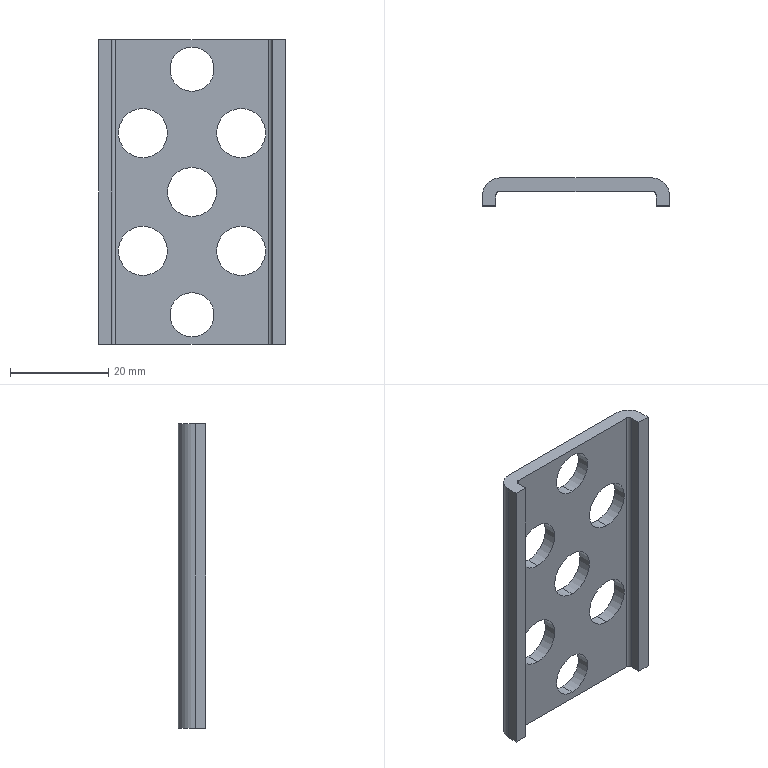Part | SolidWorks | features Fillet 2, HoleWzd 2, Extrusion 1, ICE 1 | 1 solid | 28 faces | box 37.996 x 5.595 x 62 mm | volume 5626 mm3 | cylinder 18 | plane 10 | commonest cylinder face diameters 10 x10 9 x4 1.473 x2 6.873 x2
STEP:
#1=CARTESIAN_POINT('',(0.,-2.7,-74.5));
#2=VERTEX_POINT('',#1);
#3=CARTESIAN_POINT('',(0.,-2.7,-65.5));
#4=VERTEX_POINT('',#3);
#5=CARTESIAN_POINT('',(0.,-2.7,-70.));
#6=DIRECTION('',(0.,1.,0.));
#7=DIRECTION('',(-1.,0.,0.));
#8=AXIS2_PLACEMENT_3D('',#5,#6,#7);
#9=CIRCLE('',#8,4.5);
#10=EDGE_CURVE('',#2,#4,#9,.T.);
#11=ORIENTED_EDGE('',*,*,#10,.F.);
#12=CARTESIAN_POINT('',(0.,0.,-74.5));
#13=VERTEX_POINT('',#12);
#14=CARTESIAN_POINT('',(0.,0.,-74.5));
#15=DIRECTION('',(0.,1.,0.));
#16=VECTOR('',#15,1000.);
#17=LINE('',#14,#16);
#18=EDGE_CURVE('',#2,#13,#17,.T.);
#19=ORIENTED_EDGE('',*,*,#18,.T.);
#20=CARTESIAN_POINT('',(0.,0.,-65.5));
#21=VERTEX_POINT('',#20);
#22=CARTESIAN_POINT('',(0.,0.,-70.));
#23=DIRECTION('',(0.,1.,0.));
#24=DIRECTION('',(0.,0.,1.));
#25=AXIS2_PLACEMENT_3D('',#22,#23,#24);
#26=CIRCLE('',#25,4.5);
#27=EDGE_CURVE('',#13,#21,#26,.T.);
#28=ORIENTED_EDGE('',*,*,#27,.T.);
#29=CARTESIAN_POINT('',(0.,0.,-65.5));
#30=DIRECTION('',(0.,1.,0.));
#31=VECTOR('',#30,1000.);
#32=LINE('',#29,#31);
#33=EDGE_CURVE('',#4,#21,#32,.T.);
#34=ORIENTED_EDGE('',*,*,#33,.F.);
#35=EDGE_LOOP('',(#11,#19,#28,#34));
#36=FACE_OUTER_BOUND('',#35,.T.);
#37=CARTESIAN_POINT('',(0.,0.,-70.));
#38=DIRECTION('',(0.,1.,0.));
#39=DIRECTION('',(0.,0.,1.));
#40=AXIS2_PLACEMENT_3D('',#37,#38,#39);
#41=CYLINDRICAL_SURFACE('',#40,4.5);
#42=ADVANCED_FACE('',(#36),#41,.F.);
#43=CARTESIAN_POINT('',(0.,-2.7,-24.5));
#44=VERTEX_POINT('',#43);
#45=CARTESIAN_POINT('',(0.,-2.7,-15.5));
#46=VERTEX_POINT('',#45);
#47=CARTESIAN_POINT('',(0.,-2.7,-20.));
#48=DIRECTION('',(0.,1.,0.));
#49=DIRECTION('',(-1.,0.,0.));
#50=AXIS2_PLACEMENT_3D('',#47,#48,#49);
#51=CIRCLE('',#50,4.5);
#52=EDGE_CURVE('',#44,#46,#51,.T.);
#53=ORIENTED_EDGE('',*,*,#52,.F.);
#54=CARTESIAN_POINT('',(0.,0.,-24.5));
#55=VERTEX_POINT('',#54);
#56=CARTESIAN_POINT('',(0.,0.,-24.5));
#57=DIRECTION('',(0.,1.,0.));
#58=VECTOR('',#57,1000.);
#59=LINE('',#56,#58);
#60=EDGE_CURVE('',#44,#55,#59,.T.);
#61=ORIENTED_EDGE('',*,*,#60,.T.);
#62=CARTESIAN_POINT('',(0.,0.,-15.5));
#63=VERTEX_POINT('',#62);
#64=CARTESIAN_POINT('',(0.,0.,-20.));
#65=DIRECTION('',(0.,1.,0.));
#66=DIRECTION('',(0.,0.,1.));
#67=AXIS2_PLACEMENT_3D('',#64,#65,#66);
#68=CIRCLE('',#67,4.5);
#69=EDGE_CURVE('',#55,#63,#68,.T.);
#70=ORIENTED_EDGE('',*,*,#69,.T.);
#71=CARTESIAN_POINT('',(0.,0.,-15.5));
#72=DIRECTION('',(0.,1.,0.));
#73=VECTOR('',#72,1000.);
#74=LINE('',#71,#73);
#75=EDGE_CURVE('',#46,#63,#74,.T.);
#76=ORIENTED_EDGE('',*,*,#75,.F.);
#77=EDGE_LOOP('',(#53,#61,#70,#76));
#78=FACE_OUTER_BOUND('',#77,.T.);
#79=CARTESIAN_POINT('',(0.,0.,-20.));
#80=DIRECTION('',(0.,1.,0.));
#81=DIRECTION('',(0.,0.,1.));
#82=AXIS2_PLACEMENT_3D('',#79,#80,#81);
#83=CYLINDRICAL_SURFACE('',#82,4.5);
#84=ADVANCED_FACE('',(#78),#83,.F.);
#85=CARTESIAN_POINT('',(0.,-2.7,-50.));
#86=VERTEX_POINT('',#85);
#87=CARTESIAN_POINT('',(0.,-2.7,-40.));
#88=VERTEX_POINT('',#87);
#89=CARTESIAN_POINT('',(0.,-2.7,-45.));
#90=DIRECTION('',(0.,1.,0.));
#91=DIRECTION('',(-1.,0.,0.));
#92=AXIS2_PLACEMENT_3D('',#89,#90,#91);
#93=CIRCLE('',#92,5.);
#94=EDGE_CURVE('',#86,#88,#93,.T.);
#95=ORIENTED_EDGE('',*,*,#94,.F.);
#96=CARTESIAN_POINT('',(0.,0.,-50.));
#97=VERTEX_POINT('',#96);
#98=CARTESIAN_POINT('',(0.,0.,-50.));
#99=DIRECTION('',(0.,1.,0.));
#100=VECTOR('',#99,1000.);
#101=LINE('',#98,#100);
#102=EDGE_CURVE('',#86,#97,#101,.T.);
#103=ORIENTED_EDGE('',*,*,#102,.T.);
#104=CARTESIAN_POINT('',(0.,0.,-40.));
#105=VERTEX_POINT('',#104);
#106=CARTESIAN_POINT('',(0.,0.,-45.));
#107=DIRECTION('',(0.,1.,0.));
#108=DIRECTION('',(0.,0.,1.));
#109=AXIS2_PLACEMENT_3D('',#106,#107,#108);
#110=CIRCLE('',#109,5.);
#111=EDGE_CURVE('',#97,#105,#110,.T.);
#112=ORIENTED_EDGE('',*,*,#111,.T.);
#113=CARTESIAN_POINT('',(0.,0.,-40.));
#114=DIRECTION('',(0.,1.,0.));
#115=VECTOR('',#114,1000.);
#116=LINE('',#113,#115);
#117=EDGE_CURVE('',#88,#105,#116,.T.);
#118=ORIENTED_EDGE('',*,*,#117,.F.);
#119=EDGE_LOOP('',(#95,#103,#112,#118));
#120=FACE_OUTER_BOUND('',#119,.T.);
#121=CARTESIAN_POINT('',(0.,0.,-45.));
#122=DIRECTION('',(0.,1.,0.));
#123=DIRECTION('',(0.,0.,1.));
#124=AXIS2_PLACEMENT_3D('',#121,#122,#123);
#125=CYLINDRICAL_SURFACE('',#124,5.);
#126=ADVANCED_FACE('',(#120),#125,.F.);
#127=CARTESIAN_POINT('',(-10.,-2.7,-62.));
#128=VERTEX_POINT('',#127);
#129=CARTESIAN_POINT('',(-10.,-2.7,-52.));
#130=VERTEX_POINT('',#129);
#131=CARTESIAN_POINT('',(-10.,-2.7,-57.));
#132=DIRECTION('',(0.,1.,0.));
#133=DIRECTION('',(-1.,0.,0.));
#134=AXIS2_PLACEMENT_3D('',#131,#132,#133);
#135=CIRCLE('',#134,5.);
#136=EDGE_CURVE('',#128,#130,#135,.T.);
#137=ORIENTED_EDGE('',*,*,#136,.F.);
#138=CARTESIAN_POINT('',(-10.,0.,-62.));
#139=VERTEX_POINT('',#138);
#140=CARTESIAN_POINT('',(-10.,0.,-62.));
#141=DIRECTION('',(0.,1.,0.));
#142=VECTOR('',#141,1000.);
#143=LINE('',#140,#142);
#144=EDGE_CURVE('',#128,#139,#143,.T.);
#145=ORIENTED_EDGE('',*,*,#144,.T.);
#146=CARTESIAN_POINT('',(-10.,0.,-52.));
#147=VERTEX_POINT('',#146);
#148=CARTESIAN_POINT('',(-10.,0.,-57.));
#149=DIRECTION('',(0.,1.,0.));
#150=DIRECTION('',(0.,0.,1.));
#151=AXIS2_PLACEMENT_3D('',#148,#149,#150);
#152=CIRCLE('',#151,5.);
#153=EDGE_CURVE('',#139,#147,#152,.T.);
#154=ORIENTED_EDGE('',*,*,#153,.T.);
#155=CARTESIAN_POINT('',(-10.,0.,-52.));
#156=DIRECTION('',(0.,1.,0.));
#157=VECTOR('',#156,1000.);
#158=LINE('',#155,#157);
#159=EDGE_CURVE('',#130,#147,#158,.T.);
#160=ORIENTED_EDGE('',*,*,#159,.F.);
#161=EDGE_LOOP('',(#137,#145,#154,#160));
#162=FACE_OUTER_BOUND('',#161,.T.);
#163=CARTESIAN_POINT('',(-10.,0.,-57.));
#164=DIRECTION('',(0.,1.,0.));
#165=DIRECTION('',(0.,0.,1.));
#166=AXIS2_PLACEMENT_3D('',#163,#164,#165);
#167=CYLINDRICAL_SURFACE('',#166,5.);
#168=ADVANCED_FACE('',(#162),#167,.F.);
#169=CARTESIAN_POINT('',(-10.,-2.7,-38.));
#170=VERTEX_POINT('',#169);
#171=CARTESIAN_POINT('',(-10.,-2.7,-28.));
#172=VERTEX_POINT('',#171);
#173=CARTESIAN_POINT('',(-10.,-2.7,-33.));
#174=DIRECTION('',(0.,1.,0.));
#175=DIRECTION('',(-1.,0.,0.));
#176=AXIS2_PLACEMENT_3D('',#173,#174,#175);
#177=CIRCLE('',#176,5.);
#178=EDGE_CURVE('',#170,#172,#177,.T.);
#179=ORIENTED_EDGE('',*,*,#178,.F.);
#180=CARTESIAN_POINT('',(-10.,0.,-38.));
#181=VERTEX_POINT('',#180);
#182=CARTESIAN_POINT('',(-10.,0.,-38.));
#183=DIRECTION('',(0.,1.,0.));
#184=VECTOR('',#183,1000.);
#185=LINE('',#182,#184);
#186=EDGE_CURVE('',#170,#181,#185,.T.);
#187=ORIENTED_EDGE('',*,*,#186,.T.);
#188=CARTESIAN_POINT('',(-10.,0.,-28.));
#189=VERTEX_POINT('',#188);
#190=CARTESIAN_POINT('',(-10.,0.,-33.));
#191=DIRECTION('',(0.,1.,0.));
#192=DIRECTION('',(0.,0.,1.));
#193=AXIS2_PLACEMENT_3D('',#190,#191,#192);
#194=CIRCLE('',#193,5.);
#195=EDGE_CURVE('',#181,#189,#194,.T.);
#196=ORIENTED_EDGE('',*,*,#195,.T.);
#197=CARTESIAN_POINT('',(-10.,0.,-28.));
#198=DIRECTION('',(0.,1.,0.));
#199=VECTOR('',#198,1000.);
#200=LINE('',#197,#199);
#201=EDGE_CURVE('',#172,#189,#200,.T.);
#202=ORIENTED_EDGE('',*,*,#201,.F.);
#203=EDGE_LOOP('',(#179,#187,#196,#202));
#204=FACE_OUTER_BOUND('',#203,.T.);
#205=CARTESIAN_POINT('',(-10.,0.,-33.));
#206=DIRECTION('',(0.,1.,0.));
#207=DIRECTION('',(0.,0.,1.));
#208=AXIS2_PLACEMENT_3D('',#205,#206,#207);
#209=CYLINDRICAL_SURFACE('',#208,5.);
#210=ADVANCED_FACE('',(#204),#209,.F.);
#211=CARTESIAN_POINT('',(10.,-2.7,-38.));
#212=VERTEX_POINT('',#211);
#213=CARTESIAN_POINT('',(10.,-2.7,-28.));
#214=VERTEX_POINT('',#213);
#215=CARTESIAN_POINT('',(10.,-2.7,-33.));
#216=DIRECTION('',(0.,1.,0.));
#217=DIRECTION('',(-1.,0.,0.));
#218=AXIS2_PLACEMENT_3D('',#215,#216,#217);
#219=CIRCLE('',#218,5.);
#220=EDGE_CURVE('',#212,#214,#219,.T.);
#221=ORIENTED_EDGE('',*,*,#220,.F.);
#222=CARTESIAN_POINT('',(10.,0.,-38.));
#223=VERTEX_POINT('',#222);
#224=CARTESIAN_POINT('',(10.,0.,-38.));
#225=DIRECTION('',(0.,1.,0.));
#226=VECTOR('',#225,1000.);
#227=LINE('',#224,#226);
#228=EDGE_CURVE('',#212,#223,#227,.T.);
#229=ORIENTED_EDGE('',*,*,#228,.T.);
#230=CARTESIAN_POINT('',(10.,0.,-28.));
#231=VERTEX_POINT('',#230);
#232=CARTESIAN_POINT('',(10.,0.,-33.));
#233=DIRECTION('',(0.,1.,0.));
#234=DIRECTION('',(0.,0.,1.));
#235=AXIS2_PLACEMENT_3D('',#232,#233,#234);
#236=CIRCLE('',#235,5.);
#237=EDGE_CURVE('',#223,#231,#236,.T.);
#238=ORIENTED_EDGE('',*,*,#237,.T.);
#239=CARTESIAN_POINT('',(10.,0.,-28.));
#240=DIRECTION('',(0.,1.,0.));
#241=VECTOR('',#240,1000.);
#242=LINE('',#239,#241);
#243=EDGE_CURVE('',#214,#231,#242,.T.);
#244=ORIENTED_EDGE('',*,*,#243,.F.);
#245=EDGE_LOOP('',(#221,#229,#238,#244));
#246=FACE_OUTER_BOUND('',#245,.T.);
#247=CARTESIAN_POINT('',(10.,0.,-33.));
#248=DIRECTION('',(0.,1.,0.));
#249=DIRECTION('',(0.,0.,1.));
#250=AXIS2_PLACEMENT_3D('',#247,#248,#249);
#251=CYLINDRICAL_SURFACE('',#250,5.);
#252=ADVANCED_FACE('',(#246),#251,.F.);
#253=CARTESIAN_POINT('',(10.,-2.7,-62.));
#254=VERTEX_POINT('',#253);
#255=CARTESIAN_POINT('',(10.,-2.7,-52.));
#256=VERTEX_POINT('',#255);
#257=CARTESIAN_POINT('',(10.,-2.7,-57.));
#258=DIRECTION('',(0.,1.,0.));
#259=DIRECTION('',(-1.,0.,0.));
#260=AXIS2_PLACEMENT_3D('',#257,#258,#259);
#261=CIRCLE('',#260,5.);
#262=EDGE_CURVE('',#254,#256,#261,.T.);
#263=ORIENTED_EDGE('',*,*,#262,.F.);
#264=CARTESIAN_POINT('',(10.,0.,-62.));
#265=VERTEX_POINT('',#264);
#266=CARTESIAN_POINT('',(10.,0.,-62.));
#267=DIRECTION('',(0.,1.,0.));
#268=VECTOR('',#267,1000.);
#269=LINE('',#266,#268);
#270=EDGE_CURVE('',#254,#265,#269,.T.);
#271=ORIENTED_EDGE('',*,*,#270,.T.);
#272=CARTESIAN_POINT('',(10.,0.,-52.));
#273=VERTEX_POINT('',#272);
#274=CARTESIAN_POINT('',(10.,0.,-57.));
#275=DIRECTION('',(0.,1.,0.));
#276=DIRECTION('',(0.,0.,1.));
#277=AXIS2_PLACEMENT_3D('',#274,#275,#276);
#278=CIRCLE('',#277,5.);
#279=EDGE_CURVE('',#265,#273,#278,.T.);
#280=ORIENTED_EDGE('',*,*,#279,.T.);
#281=CARTESIAN_POINT('',(10.,0.,-52.));
#282=DIRECTION('',(0.,1.,0.));
#283=VECTOR('',#282,1000.);
#284=LINE('',#281,#283);
#285=EDGE_CURVE('',#256,#273,#284,.T.);
#286=ORIENTED_EDGE('',*,*,#285,.F.);
#287=EDGE_LOOP('',(#263,#271,#280,#286));
#288=FACE_OUTER_BOUND('',#287,.T.);
#289=CARTESIAN_POINT('',(10.,0.,-57.));
#290=DIRECTION('',(0.,1.,0.));
#291=DIRECTION('',(0.,0.,1.));
#292=AXIS2_PLACEMENT_3D('',#289,#290,#291);
#293=CYLINDRICAL_SURFACE('',#292,5.);
#294=ADVANCED_FACE('',(#288),#293,.F.);
#295=CARTESIAN_POINT('',(16.298,-5.595,-14.));
#296=VERTEX_POINT('',#295);
#297=CARTESIAN_POINT('',(18.998,-5.595,-14.));
#298=VERTEX_POINT('',#297);
#299=CARTESIAN_POINT('',(-18.998,-5.595,-14.));
#300=DIRECTION('',(1.,0.,0.));
#301=VECTOR('',#300,1000.);
#302=LINE('',#299,#301);
#303=EDGE_CURVE('',#296,#298,#302,.T.);
#304=ORIENTED_EDGE('',*,*,#303,.F.);
#305=CARTESIAN_POINT('',(16.298,-5.595,-76.));
#306=VERTEX_POINT('',#305);
#307=CARTESIAN_POINT('',(16.298,-5.595,-14.));
#308=DIRECTION('',(0.,0.,-1.));
#309=VECTOR('',#308,1000.);
#310=LINE('',#307,#309);
#311=EDGE_CURVE('',#296,#306,#310,.T.);
#312=ORIENTED_EDGE('',*,*,#311,.T.);
#313=CARTESIAN_POINT('',(18.998,-5.595,-76.));
#314=VERTEX_POINT('',#313);
#315=CARTESIAN_POINT('',(18.998,-5.595,-76.));
#316=DIRECTION('',(-1.,0.,0.));
#317=VECTOR('',#316,1000.);
#318=LINE('',#315,#317);
#319=EDGE_CURVE('',#314,#306,#318,.T.);
#320=ORIENTED_EDGE('',*,*,#319,.F.);
#321=CARTESIAN_POINT('',(18.998,-5.595,-14.));
#322=DIRECTION('',(0.,0.,-1.));
#323=VECTOR('',#322,1000.);
#324=LINE('',#321,#323);
#325=EDGE_CURVE('',#298,#314,#324,.T.);
#326=ORIENTED_EDGE('',*,*,#325,.F.);
#327=EDGE_LOOP('',(#304,#312,#320,#326));
#328=FACE_OUTER_BOUND('',#327,.T.);
#329=CARTESIAN_POINT('',(0.,-5.595,0.));
#330=DIRECTION('',(0.,1.,0.));
#331=DIRECTION('',(0.,0.,1.));
#332=AXIS2_PLACEMENT_3D('',#329,#330,#331);
#333=PLANE('',#332);
#334=ADVANCED_FACE('',(#328),#333,.F.);
#335=CARTESIAN_POINT('',(-18.998,-5.595,-14.));
#336=VERTEX_POINT('',#335);
#337=CARTESIAN_POINT('',(-18.998,-3.437,-14.));
#338=VERTEX_POINT('',#337);
#339=CARTESIAN_POINT('',(-18.998,-5.595,-14.));
#340=DIRECTION('',(0.,1.,0.));
#341=VECTOR('',#340,1000.);
#342=LINE('',#339,#341);
#343=EDGE_CURVE('',#336,#338,#342,.T.);
#344=ORIENTED_EDGE('',*,*,#343,.T.);
#345=CARTESIAN_POINT('',(-18.998,-3.437,-76.));
#346=VERTEX_POINT('',#345);
#347=CARTESIAN_POINT('',(-18.998,-3.437,-76.));
#348=DIRECTION('',(0.,0.,-1.));
#349=VECTOR('',#348,1000.);
#350=LINE('',#347,#349);
#351=EDGE_CURVE('',#338,#346,#350,.T.);
#352=ORIENTED_EDGE('',*,*,#351,.T.);
#353=CARTESIAN_POINT('',(-18.998,-5.595,-76.));
#354=VERTEX_POINT('',#353);
#355=CARTESIAN_POINT('',(-18.998,-5.595,-76.));
#356=DIRECTION('',(0.,1.,0.));
#357=VECTOR('',#356,1000.);
#358=LINE('',#355,#357);
#359=EDGE_CURVE('',#354,#346,#358,.T.);
#360=ORIENTED_EDGE('',*,*,#359,.F.);
#361=CARTESIAN_POINT('',(-18.998,-5.595,-76.));
#362=DIRECTION('',(0.,0.,1.));
#363=VECTOR('',#362,1000.);
#364=LINE('',#361,#363);
#365=EDGE_CURVE('',#354,#336,#364,.T.);
#366=ORIENTED_EDGE('',*,*,#365,.T.);
#367=EDGE_LOOP('',(#344,#352,#360,#366));
#368=FACE_OUTER_BOUND('',#367,.T.);
#369=CARTESIAN_POINT('',(-18.998,-5.595,-76.));
#370=DIRECTION('',(-1.,0.,0.));
#371=DIRECTION('',(0.,0.,1.));
#372=AXIS2_PLACEMENT_3D('',#369,#370,#371);
#373=PLANE('',#372);
#374=ADVANCED_FACE('',(#368),#373,.T.);
#375=CARTESIAN_POINT('',(15.561,0.,-76.));
#376=VERTEX_POINT('',#375);
#377=CARTESIAN_POINT('',(-15.561,0.,-76.));
#378=VERTEX_POINT('',#377);
#379=CARTESIAN_POINT('',(18.998,0.,-76.));
#380=DIRECTION('',(-1.,0.,0.));
#381=VECTOR('',#380,1000.);
#382=LINE('',#379,#381);
#383=EDGE_CURVE('',#376,#378,#382,.T.);
#384=ORIENTED_EDGE('',*,*,#383,.F.);
#385=CARTESIAN_POINT('',(18.998,-3.437,-76.));
#386=VERTEX_POINT('',#385);
#387=CARTESIAN_POINT('',(15.561,-3.437,-76.));
#388=DIRECTION('',(0.,0.,-1.));
#389=DIRECTION('',(-1.,0.,0.));
#390=AXIS2_PLACEMENT_3D('',#387,#388,#389);
#391=CIRCLE('',#390,3.437);
#392=EDGE_CURVE('',#376,#386,#391,.T.);
#393=ORIENTED_EDGE('',*,*,#392,.T.);
#394=CARTESIAN_POINT('',(18.998,-5.595,-76.));
#395=DIRECTION('',(0.,1.,0.));
#396=VECTOR('',#395,1000.);
#397=LINE('',#394,#396);
#398=EDGE_CURVE('',#314,#386,#397,.T.);
#399=ORIENTED_EDGE('',*,*,#398,.F.);
#400=ORIENTED_EDGE('',*,*,#319,.T.);
#401=CARTESIAN_POINT('',(16.298,-3.437,-76.));
#402=VERTEX_POINT('',#401);
#403=CARTESIAN_POINT('',(16.298,-2.7,-76.));
#404=DIRECTION('',(0.,-1.,0.));
#405=VECTOR('',#404,1000.);
#406=LINE('',#403,#405);
#407=EDGE_CURVE('',#402,#306,#406,.T.);
#408=ORIENTED_EDGE('',*,*,#407,.F.);
#409=CARTESIAN_POINT('',(15.561,-2.7,-76.));
#410=VERTEX_POINT('',#409);
#411=CARTESIAN_POINT('',(15.561,-3.437,-76.));
#412=DIRECTION('',(0.,0.,1.));
#413=DIRECTION('',(-1.,0.,0.));
#414=AXIS2_PLACEMENT_3D('',#411,#412,#413);
#415=CIRCLE('',#414,0.7366);
#416=EDGE_CURVE('',#402,#410,#415,.T.);
#417=ORIENTED_EDGE('',*,*,#416,.T.);
#418=CARTESIAN_POINT('',(-15.561,-2.7,-76.));
#419=VERTEX_POINT('',#418);
#420=CARTESIAN_POINT('',(-16.298,-2.7,-76.));
#421=DIRECTION('',(1.,0.,0.));
#422=VECTOR('',#421,1000.);
#423=LINE('',#420,#422);
#424=EDGE_CURVE('',#419,#410,#423,.T.);
#425=ORIENTED_EDGE('',*,*,#424,.F.);
#426=CARTESIAN_POINT('',(-16.298,-3.437,-76.));
#427=VERTEX_POINT('',#426);
#428=CARTESIAN_POINT('',(-15.561,-3.437,-76.));
#429=DIRECTION('',(0.,0.,1.));
#430=DIRECTION('',(-1.,0.,0.));
#431=AXIS2_PLACEMENT_3D('',#428,#429,#430);
#432=CIRCLE('',#431,0.7366);
#433=EDGE_CURVE('',#419,#427,#432,.T.);
#434=ORIENTED_EDGE('',*,*,#433,.T.);
#435=CARTESIAN_POINT('',(-16.298,-5.595,-76.));
#436=VERTEX_POINT('',#435);
#437=CARTESIAN_POINT('',(-16.298,-5.595,-76.));
#438=DIRECTION('',(0.,1.,0.));
#439=VECTOR('',#438,1000.);
#440=LINE('',#437,#439);
#441=EDGE_CURVE('',#436,#427,#440,.T.);
#442=ORIENTED_EDGE('',*,*,#441,.F.);
#443=CARTESIAN_POINT('',(18.998,-5.595,-76.));
#444=DIRECTION('',(-1.,0.,0.));
#445=VECTOR('',#444,1000.);
#446=LINE('',#443,#445);
#447=EDGE_CURVE('',#436,#354,#446,.T.);
#448=ORIENTED_EDGE('',*,*,#447,.T.);
#449=ORIENTED_EDGE('',*,*,#359,.T.);
#450=CARTESIAN_POINT('',(-15.561,-3.437,-76.));
#451=DIRECTION('',(0.,0.,-1.));
#452=DIRECTION('',(-1.,0.,0.));
#453=AXIS2_PLACEMENT_3D('',#450,#451,#452);
#454=CIRCLE('',#453,3.437);
#455=EDGE_CURVE('',#346,#378,#454,.T.);
#456=ORIENTED_EDGE('',*,*,#455,.T.);
#457=EDGE_LOOP('',(#384,#393,#399,#400,#408,#417,#425,#434,#442,#448,#449,#456));
#458=FACE_OUTER_BOUND('',#457,.T.);
#459=CARTESIAN_POINT('',(18.998,-5.595,-76.));
#460=DIRECTION('',(0.,0.,-1.));
#461=DIRECTION('',(-1.,0.,0.));
#462=AXIS2_PLACEMENT_3D('',#459,#460,#461);
#463=PLANE('',#462);
#464=ADVANCED_FACE('',(#458),#463,.T.);
#465=ORIENTED_EDGE('',*,*,#398,.T.);
#466=CARTESIAN_POINT('',(18.998,-3.437,-14.));
#467=VERTEX_POINT('',#466);
#468=CARTESIAN_POINT('',(18.998,-3.437,-14.));
#469=DIRECTION('',(0.,0.,1.));
#470=VECTOR('',#469,1000.);
#471=LINE('',#468,#470);
#472=EDGE_CURVE('',#386,#467,#471,.T.);
#473=ORIENTED_EDGE('',*,*,#472,.T.);
#474=CARTESIAN_POINT('',(18.998,-5.595,-14.));
#475=DIRECTION('',(0.,1.,0.));
#476=VECTOR('',#475,1000.);
#477=LINE('',#474,#476);
#478=EDGE_CURVE('',#298,#467,#477,.T.);
#479=ORIENTED_EDGE('',*,*,#478,.F.);
#480=ORIENTED_EDGE('',*,*,#325,.T.);
#481=EDGE_LOOP('',(#465,#473,#479,#480));
#482=FACE_OUTER_BOUND('',#481,.T.);
#483=CARTESIAN_POINT('',(18.998,-5.595,-14.));
#484=DIRECTION('',(1.,0.,0.));
#485=DIRECTION('',(0.,0.,-1.));
#486=AXIS2_PLACEMENT_3D('',#483,#484,#485);
#487=PLANE('',#486);
#488=ADVANCED_FACE('',(#482),#487,.T.);
#489=ORIENTED_EDGE('',*,*,#478,.T.);
#490=CARTESIAN_POINT('',(15.561,0.,-14.));
#491=VERTEX_POINT('',#490);
#492=CARTESIAN_POINT('',(15.561,-3.437,-14.));
#493=DIRECTION('',(0.,0.,1.));
#494=DIRECTION('',(1.,0.,0.));
#495=AXIS2_PLACEMENT_3D('',#492,#493,#494);
#496=CIRCLE('',#495,3.437);
#497=EDGE_CURVE('',#467,#491,#496,.T.);
#498=ORIENTED_EDGE('',*,*,#497,.T.);
#499=CARTESIAN_POINT('',(-15.561,0.,-14.));
#500=VERTEX_POINT('',#499);
#501=CARTESIAN_POINT('',(-18.998,0.,-14.));
#502=DIRECTION('',(1.,0.,0.));
#503=VECTOR('',#502,1000.);
#504=LINE('',#501,#503);
#505=EDGE_CURVE('',#500,#491,#504,.T.);
#506=ORIENTED_EDGE('',*,*,#505,.F.);
#507=CARTESIAN_POINT('',(-15.561,-3.437,-14.));
#508=DIRECTION('',(0.,0.,1.));
#509=DIRECTION('',(1.,0.,0.));
#510=AXIS2_PLACEMENT_3D('',#507,#508,#509);
#511=CIRCLE('',#510,3.437);
#512=EDGE_CURVE('',#500,#338,#511,.T.);
#513=ORIENTED_EDGE('',*,*,#512,.T.);
#514=ORIENTED_EDGE('',*,*,#343,.F.);
#515=CARTESIAN_POINT('',(-16.298,-5.595,-14.));
#516=VERTEX_POINT('',#515);
#517=CARTESIAN_POINT('',(-18.998,-5.595,-14.));
#518=DIRECTION('',(1.,0.,0.));
#519=VECTOR('',#518,1000.);
#520=LINE('',#517,#519);
#521=EDGE_CURVE('',#336,#516,#520,.T.);
#522=ORIENTED_EDGE('',*,*,#521,.T.);
#523=CARTESIAN_POINT('',(-16.298,-3.437,-14.));
#524=VERTEX_POINT('',#523);
#525=CARTESIAN_POINT('',(-16.298,-5.595,-14.));
#526=DIRECTION('',(0.,1.,0.));
#527=VECTOR('',#526,1000.);
#528=LINE('',#525,#527);
#529=EDGE_CURVE('',#516,#524,#528,.T.);
#530=ORIENTED_EDGE('',*,*,#529,.T.);
#531=CARTESIAN_POINT('',(-15.561,-2.7,-14.));
#532=VERTEX_POINT('',#531);
#533=CARTESIAN_POINT('',(-15.561,-3.437,-14.));
#534=DIRECTION('',(0.,0.,-1.));
#535=DIRECTION('',(1.,0.,0.));
#536=AXIS2_PLACEMENT_3D('',#533,#534,#535);
#537=CIRCLE('',#536,0.7366);
#538=EDGE_CURVE('',#524,#532,#537,.T.);
#539=ORIENTED_EDGE('',*,*,#538,.T.);
#540=CARTESIAN_POINT('',(15.561,-2.7,-14.));
#541=VERTEX_POINT('',#540);
#542=CARTESIAN_POINT('',(-16.298,-2.7,-14.));
#543=DIRECTION('',(1.,0.,0.));
#544=VECTOR('',#543,1000.);
#545=LINE('',#542,#544);
#546=EDGE_CURVE('',#532,#541,#545,.T.);
#547=ORIENTED_EDGE('',*,*,#546,.T.);
#548=CARTESIAN_POINT('',(16.298,-3.437,-14.));
#549=VERTEX_POINT('',#548);
#550=CARTESIAN_POINT('',(15.561,-3.437,-14.));
#551=DIRECTION('',(0.,0.,-1.));
#552=DIRECTION('',(1.,0.,0.));
#553=AXIS2_PLACEMENT_3D('',#550,#551,#552);
#554=CIRCLE('',#553,0.7366);
#555=EDGE_CURVE('',#541,#549,#554,.T.);
#556=ORIENTED_EDGE('',*,*,#555,.T.);
#557=CARTESIAN_POINT('',(16.298,-2.7,-14.));
#558=DIRECTION('',(0.,-1.,0.));
#559=VECTOR('',#558,1000.);
#560=LINE('',#557,#559);
#561=EDGE_CURVE('',#549,#296,#560,.T.);
#562=ORIENTED_EDGE('',*,*,#561,.T.);
#563=ORIENTED_EDGE('',*,*,#303,.T.);
#564=EDGE_LOOP('',(#489,#498,#506,#513,#514,#522,#530,#539,#547,#556,#562,#563));
#565=FACE_OUTER_BOUND('',#564,.T.);
#566=CARTESIAN_POINT('',(-18.998,-5.595,-14.));
#567=DIRECTION('',(0.,0.,1.));
#568=DIRECTION('',(1.,0.,0.));
#569=AXIS2_PLACEMENT_3D('',#566,#567,#568);
#570=PLANE('',#569);
#571=ADVANCED_FACE('',(#565),#570,.T.);
#572=ORIENTED_EDGE('',*,*,#447,.F.);
#573=CARTESIAN_POINT('',(-16.298,-5.595,-14.));
#574=DIRECTION('',(0.,0.,-1.));
#575=VECTOR('',#574,1000.);
#576=LINE('',#573,#575);
#577=EDGE_CURVE('',#516,#436,#576,.T.);
#578=ORIENTED_EDGE('',*,*,#577,.F.);
#579=ORIENTED_EDGE('',*,*,#521,.F.);
#580=ORIENTED_EDGE('',*,*,#365,.F.);
#581=EDGE_LOOP('',(#572,#578,#579,#580));
#582=FACE_OUTER_BOUND('',#581,.T.);
#583=CARTESIAN_POINT('',(0.,-5.595,0.));
#584=DIRECTION('',(0.,1.,0.));
#585=DIRECTION('',(0.,0.,1.));
#586=AXIS2_PLACEMENT_3D('',#583,#584,#585);
#587=PLANE('',#586);
#588=ADVANCED_FACE('',(#582),#587,.F.);
#589=CARTESIAN_POINT('',(0.,0.,-70.));
#590=DIRECTION('',(0.,1.,0.));
#591=DIRECTION('',(0.,0.,1.));
#592=AXIS2_PLACEMENT_3D('',#589,#590,#591);
#593=CIRCLE('',#592,4.5);
#594=EDGE_CURVE('',#21,#13,#593,.T.);
#595=ORIENTED_EDGE('',*,*,#594,.F.);
#596=ORIENTED_EDGE('',*,*,#27,.F.);
#597=EDGE_LOOP('',(#595,#596));
#598=FACE_BOUND('',#597,.T.);
#599=CARTESIAN_POINT('',(0.,0.,-20.));
#600=DIRECTION('',(0.,1.,0.));
#601=DIRECTION('',(0.,0.,1.));
#602=AXIS2_PLACEMENT_3D('',#599,#600,#601);
#603=CIRCLE('',#602,4.5);
#604=EDGE_CURVE('',#63,#55,#603,.T.);
#605=ORIENTED_EDGE('',*,*,#604,.F.);
#606=ORIENTED_EDGE('',*,*,#69,.F.);
#607=EDGE_LOOP('',(#605,#606));
#608=FACE_BOUND('',#607,.T.);
#609=CARTESIAN_POINT('',(0.,0.,-45.));
#610=DIRECTION('',(0.,1.,0.));
#611=DIRECTION('',(0.,0.,1.));
#612=AXIS2_PLACEMENT_3D('',#609,#610,#611);
#613=CIRCLE('',#612,5.);
#614=EDGE_CURVE('',#105,#97,#613,.T.);
#615=ORIENTED_EDGE('',*,*,#614,.F.);
#616=ORIENTED_EDGE('',*,*,#111,.F.);
#617=EDGE_LOOP('',(#615,#616));
#618=FACE_BOUND('',#617,.T.);
#619=CARTESIAN_POINT('',(-10.,0.,-57.));
#620=DIRECTION('',(0.,1.,0.));
#621=DIRECTION('',(0.,0.,1.));
#622=AXIS2_PLACEMENT_3D('',#619,#620,#621);
#623=CIRCLE('',#622,5.);
#624=EDGE_CURVE('',#147,#139,#623,.T.);
#625=ORIENTED_EDGE('',*,*,#624,.F.);
#626=ORIENTED_EDGE('',*,*,#153,.F.);
#627=EDGE_LOOP('',(#625,#626));
#628=FACE_BOUND('',#627,.T.);
#629=CARTESIAN_POINT('',(-10.,0.,-33.));
#630=DIRECTION('',(0.,1.,0.));
#631=DIRECTION('',(0.,0.,1.));
#632=AXIS2_PLACEMENT_3D('',#629,#630,#631);
#633=CIRCLE('',#632,5.);
#634=EDGE_CURVE('',#189,#181,#633,.T.);
#635=ORIENTED_EDGE('',*,*,#634,.F.);
#636=ORIENTED_EDGE('',*,*,#195,.F.);
#637=EDGE_LOOP('',(#635,#636));
#638=FACE_BOUND('',#637,.T.);
#639=CARTESIAN_POINT('',(10.,0.,-33.));
#640=DIRECTION('',(0.,1.,0.));
#641=DIRECTION('',(0.,0.,1.));
#642=AXIS2_PLACEMENT_3D('',#639,#640,#641);
#643=CIRCLE('',#642,5.);
#644=EDGE_CURVE('',#231,#223,#643,.T.);
#645=ORIENTED_EDGE('',*,*,#644,.F.);
#646=ORIENTED_EDGE('',*,*,#237,.F.);
#647=EDGE_LOOP('',(#645,#646));
#648=FACE_BOUND('',#647,.T.);
#649=CARTESIAN_POINT('',(10.,0.,-57.));
#650=DIRECTION('',(0.,1.,0.));
#651=DIRECTION('',(0.,0.,1.));
#652=AXIS2_PLACEMENT_3D('',#649,#650,#651);
#653=CIRCLE('',#652,5.);
#654=EDGE_CURVE('',#273,#265,#653,.T.);
#655=ORIENTED_EDGE('',*,*,#654,.F.);
#656=ORIENTED_EDGE('',*,*,#279,.F.);
#657=EDGE_LOOP('',(#655,#656));
#658=FACE_BOUND('',#657,.T.);
#659=ORIENTED_EDGE('',*,*,#505,.T.);
#660=CARTESIAN_POINT('',(15.561,0.,0.));
#661=DIRECTION('',(0.,0.,-1.));
#662=VECTOR('',#661,1000.);
#663=LINE('',#660,#662);
#664=EDGE_CURVE('',#491,#376,#663,.T.);
#665=ORIENTED_EDGE('',*,*,#664,.T.);
#666=ORIENTED_EDGE('',*,*,#383,.T.);
#667=CARTESIAN_POINT('',(-15.561,0.,0.));
#668=DIRECTION('',(0.,0.,1.));
#669=VECTOR('',#668,1000.);
#670=LINE('',#667,#669);
#671=EDGE_CURVE('',#378,#500,#670,.T.);
#672=ORIENTED_EDGE('',*,*,#671,.T.);
#673=EDGE_LOOP('',(#659,#665,#666,#672));
#674=FACE_OUTER_BOUND('',#673,.T.);
#675=CARTESIAN_POINT('',(0.,0.,0.));
#676=DIRECTION('',(0.,1.,0.));
#677=DIRECTION('',(0.,0.,1.));
#678=AXIS2_PLACEMENT_3D('',#675,#676,#677);
#679=PLANE('',#678);
#680=ADVANCED_FACE('',(#598,#608,#618,#628,#638,#648,#658,#674),#679,.T.);
#681=ORIENTED_EDGE('',*,*,#561,.F.);
#682=CARTESIAN_POINT('',(16.298,-3.437,-76.));
#683=DIRECTION('',(0.,0.,-1.));
#684=VECTOR('',#683,1000.);
#685=LINE('',#682,#684);
#686=EDGE_CURVE('',#549,#402,#685,.T.);
#687=ORIENTED_EDGE('',*,*,#686,.T.);
#688=ORIENTED_EDGE('',*,*,#407,.T.);
#689=ORIENTED_EDGE('',*,*,#311,.F.);
#690=EDGE_LOOP('',(#681,#687,#688,#689));
#691=FACE_OUTER_BOUND('',#690,.T.);
#692=CARTESIAN_POINT('',(16.298,-2.7,-14.));
#693=DIRECTION('',(1.,0.,0.));
#694=DIRECTION('',(0.,1.,0.));
#695=AXIS2_PLACEMENT_3D('',#692,#693,#694);
#696=PLANE('',#695);
#697=ADVANCED_FACE('',(#691),#696,.F.);
#698=CARTESIAN_POINT('',(0.,-2.7,-70.));
#699=DIRECTION('',(0.,1.,0.));
#700=DIRECTION('',(-1.,0.,0.));
#701=AXIS2_PLACEMENT_3D('',#698,#699,#700);
#702=CIRCLE('',#701,4.5);
#703=EDGE_CURVE('',#4,#2,#702,.T.);
#704=ORIENTED_EDGE('',*,*,#703,.T.);
#705=ORIENTED_EDGE('',*,*,#10,.T.);
#706=EDGE_LOOP('',(#704,#705));
#707=FACE_BOUND('',#706,.T.);
#708=CARTESIAN_POINT('',(0.,-2.7,-20.));
#709=DIRECTION('',(0.,1.,0.));
#710=DIRECTION('',(-1.,0.,0.));
#711=AXIS2_PLACEMENT_3D('',#708,#709,#710);
#712=CIRCLE('',#711,4.5);
#713=EDGE_CURVE('',#46,#44,#712,.T.);
#714=ORIENTED_EDGE('',*,*,#713,.T.);
#715=ORIENTED_EDGE('',*,*,#52,.T.);
#716=EDGE_LOOP('',(#714,#715));
#717=FACE_BOUND('',#716,.T.);
#718=CARTESIAN_POINT('',(0.,-2.7,-45.));
#719=DIRECTION('',(0.,1.,0.));
#720=DIRECTION('',(-1.,0.,0.));
#721=AXIS2_PLACEMENT_3D('',#718,#719,#720);
#722=CIRCLE('',#721,5.);
#723=EDGE_CURVE('',#88,#86,#722,.T.);
#724=ORIENTED_EDGE('',*,*,#723,.T.);
#725=ORIENTED_EDGE('',*,*,#94,.T.);
#726=EDGE_LOOP('',(#724,#725));
#727=FACE_BOUND('',#726,.T.);
#728=CARTESIAN_POINT('',(-10.,-2.7,-57.));
#729=DIRECTION('',(0.,1.,0.));
#730=DIRECTION('',(-1.,0.,0.));
#731=AXIS2_PLACEMENT_3D('',#728,#729,#730);
#732=CIRCLE('',#731,5.);
#733=EDGE_CURVE('',#130,#128,#732,.T.);
#734=ORIENTED_EDGE('',*,*,#733,.T.);
#735=ORIENTED_EDGE('',*,*,#136,.T.);
#736=EDGE_LOOP('',(#734,#735));
#737=FACE_BOUND('',#736,.T.);
#738=CARTESIAN_POINT('',(-10.,-2.7,-33.));
#739=DIRECTION('',(0.,1.,0.));
#740=DIRECTION('',(-1.,0.,0.));
#741=AXIS2_PLACEMENT_3D('',#738,#739,#740);
#742=CIRCLE('',#741,5.);
#743=EDGE_CURVE('',#172,#170,#742,.T.);
#744=ORIENTED_EDGE('',*,*,#743,.T.);
#745=ORIENTED_EDGE('',*,*,#178,.T.);
#746=EDGE_LOOP('',(#744,#745));
#747=FACE_BOUND('',#746,.T.);
#748=CARTESIAN_POINT('',(10.,-2.7,-33.));
#749=DIRECTION('',(0.,1.,0.));
#750=DIRECTION('',(-1.,0.,0.));
#751=AXIS2_PLACEMENT_3D('',#748,#749,#750);
#752=CIRCLE('',#751,5.);
#753=EDGE_CURVE('',#214,#212,#752,.T.);
#754=ORIENTED_EDGE('',*,*,#753,.T.);
#755=ORIENTED_EDGE('',*,*,#220,.T.);
#756=EDGE_LOOP('',(#754,#755));
#757=FACE_BOUND('',#756,.T.);
#758=CARTESIAN_POINT('',(10.,-2.7,-57.));
#759=DIRECTION('',(0.,1.,0.));
#760=DIRECTION('',(-1.,0.,0.));
#761=AXIS2_PLACEMENT_3D('',#758,#759,#760);
#762=CIRCLE('',#761,5.);
#763=EDGE_CURVE('',#256,#254,#762,.T.);
#764=ORIENTED_EDGE('',*,*,#763,.T.);
#765=ORIENTED_EDGE('',*,*,#262,.T.);
#766=EDGE_LOOP('',(#764,#765));
#767=FACE_BOUND('',#766,.T.);
#768=ORIENTED_EDGE('',*,*,#546,.F.);
#769=CARTESIAN_POINT('',(-15.561,-2.7,-76.));
#770=DIRECTION('',(0.,0.,-1.));
#771=VECTOR('',#770,1000.);
#772=LINE('',#769,#771);
#773=EDGE_CURVE('',#532,#419,#772,.T.);
#774=ORIENTED_EDGE('',*,*,#773,.T.);
#775=ORIENTED_EDGE('',*,*,#424,.T.);
#776=CARTESIAN_POINT('',(15.561,-2.7,-14.));
#777=DIRECTION('',(0.,0.,1.));
#778=VECTOR('',#777,1000.);
#779=LINE('',#776,#778);
#780=EDGE_CURVE('',#410,#541,#779,.T.);
#781=ORIENTED_EDGE('',*,*,#780,.T.);
#782=EDGE_LOOP('',(#768,#774,#775,#781));
#783=FACE_OUTER_BOUND('',#782,.T.);
#784=CARTESIAN_POINT('',(-16.298,-2.7,-14.));
#785=DIRECTION('',(0.,1.,0.));
#786=DIRECTION('',(-1.,0.,0.));
#787=AXIS2_PLACEMENT_3D('',#784,#785,#786);
#788=PLANE('',#787);
#789=ADVANCED_FACE('',(#707,#717,#727,#737,#747,#757,#767,#783),#788,.F.);
#790=ORIENTED_EDGE('',*,*,#441,.T.);
#791=CARTESIAN_POINT('',(-16.298,-3.437,-14.));
#792=DIRECTION('',(0.,0.,1.));
#793=VECTOR('',#792,1000.);
#794=LINE('',#791,#793);
#795=EDGE_CURVE('',#427,#524,#794,.T.);
#796=ORIENTED_EDGE('',*,*,#795,.T.);
#797=ORIENTED_EDGE('',*,*,#529,.F.);
#798=ORIENTED_EDGE('',*,*,#577,.T.);
#799=EDGE_LOOP('',(#790,#796,#797,#798));
#800=FACE_OUTER_BOUND('',#799,.T.);
#801=CARTESIAN_POINT('',(-16.298,-5.595,-14.));
#802=DIRECTION('',(-1.,0.,0.));
#803=DIRECTION('',(0.,-1.,0.));
#804=AXIS2_PLACEMENT_3D('',#801,#802,#803);
#805=PLANE('',#804);
#806=ADVANCED_FACE('',(#800),#805,.F.);
#807=ORIENTED_EDGE('',*,*,#270,.F.);
#808=ORIENTED_EDGE('',*,*,#763,.F.);
#809=ORIENTED_EDGE('',*,*,#285,.T.);
#810=ORIENTED_EDGE('',*,*,#654,.T.);
#811=EDGE_LOOP('',(#807,#808,#809,#810));
#812=FACE_OUTER_BOUND('',#811,.T.);
#813=CARTESIAN_POINT('',(10.,0.,-57.));
#814=DIRECTION('',(0.,1.,0.));
#815=DIRECTION('',(0.,0.,1.));
#816=AXIS2_PLACEMENT_3D('',#813,#814,#815);
#817=CYLINDRICAL_SURFACE('',#816,5.);
#818=ADVANCED_FACE('',(#812),#817,.F.);
#819=ORIENTED_EDGE('',*,*,#228,.F.);
#820=ORIENTED_EDGE('',*,*,#753,.F.);
#821=ORIENTED_EDGE('',*,*,#243,.T.);
#822=ORIENTED_EDGE('',*,*,#644,.T.);
#823=EDGE_LOOP('',(#819,#820,#821,#822));
#824=FACE_OUTER_BOUND('',#823,.T.);
#825=CARTESIAN_POINT('',(10.,0.,-33.));
#826=DIRECTION('',(0.,1.,0.));
#827=DIRECTION('',(0.,0.,1.));
#828=AXIS2_PLACEMENT_3D('',#825,#826,#827);
#829=CYLINDRICAL_SURFACE('',#828,5.);
#830=ADVANCED_FACE('',(#824),#829,.F.);
#831=ORIENTED_EDGE('',*,*,#186,.F.);
#832=ORIENTED_EDGE('',*,*,#743,.F.);
#833=ORIENTED_EDGE('',*,*,#201,.T.);
#834=ORIENTED_EDGE('',*,*,#634,.T.);
#835=EDGE_LOOP('',(#831,#832,#833,#834));
#836=FACE_OUTER_BOUND('',#835,.T.);
#837=CARTESIAN_POINT('',(-10.,0.,-33.));
#838=DIRECTION('',(0.,1.,0.));
#839=DIRECTION('',(0.,0.,1.));
#840=AXIS2_PLACEMENT_3D('',#837,#838,#839);
#841=CYLINDRICAL_SURFACE('',#840,5.);
#842=ADVANCED_FACE('',(#836),#841,.F.);
#843=ORIENTED_EDGE('',*,*,#144,.F.);
#844=ORIENTED_EDGE('',*,*,#733,.F.);
#845=ORIENTED_EDGE('',*,*,#159,.T.);
#846=ORIENTED_EDGE('',*,*,#624,.T.);
#847=EDGE_LOOP('',(#843,#844,#845,#846));
#848=FACE_OUTER_BOUND('',#847,.T.);
#849=CARTESIAN_POINT('',(-10.,0.,-57.));
#850=DIRECTION('',(0.,1.,0.));
#851=DIRECTION('',(0.,0.,1.));
#852=AXIS2_PLACEMENT_3D('',#849,#850,#851);
#853=CYLINDRICAL_SURFACE('',#852,5.);
#854=ADVANCED_FACE('',(#848),#853,.F.);
#855=ORIENTED_EDGE('',*,*,#102,.F.);
#856=ORIENTED_EDGE('',*,*,#723,.F.);
#857=ORIENTED_EDGE('',*,*,#117,.T.);
#858=ORIENTED_EDGE('',*,*,#614,.T.);
#859=EDGE_LOOP('',(#855,#856,#857,#858));
#860=FACE_OUTER_BOUND('',#859,.T.);
#861=CARTESIAN_POINT('',(0.,0.,-45.));
#862=DIRECTION('',(0.,1.,0.));
#863=DIRECTION('',(0.,0.,1.));
#864=AXIS2_PLACEMENT_3D('',#861,#862,#863);
#865=CYLINDRICAL_SURFACE('',#864,5.);
#866=ADVANCED_FACE('',(#860),#865,.F.);
#867=ORIENTED_EDGE('',*,*,#60,.F.);
#868=ORIENTED_EDGE('',*,*,#713,.F.);
#869=ORIENTED_EDGE('',*,*,#75,.T.);
#870=ORIENTED_EDGE('',*,*,#604,.T.);
#871=EDGE_LOOP('',(#867,#868,#869,#870));
#872=FACE_OUTER_BOUND('',#871,.T.);
#873=CARTESIAN_POINT('',(0.,0.,-20.));
#874=DIRECTION('',(0.,1.,0.));
#875=DIRECTION('',(0.,0.,1.));
#876=AXIS2_PLACEMENT_3D('',#873,#874,#875);
#877=CYLINDRICAL_SURFACE('',#876,4.5);
#878=ADVANCED_FACE('',(#872),#877,.F.);
#879=ORIENTED_EDGE('',*,*,#18,.F.);
#880=ORIENTED_EDGE('',*,*,#703,.F.);
#881=ORIENTED_EDGE('',*,*,#33,.T.);
#882=ORIENTED_EDGE('',*,*,#594,.T.);
#883=EDGE_LOOP('',(#879,#880,#881,#882));
#884=FACE_OUTER_BOUND('',#883,.T.);
#885=CARTESIAN_POINT('',(0.,0.,-70.));
#886=DIRECTION('',(0.,1.,0.));
#887=DIRECTION('',(0.,0.,1.));
#888=AXIS2_PLACEMENT_3D('',#885,#886,#887);
#889=CYLINDRICAL_SURFACE('',#888,4.5);
#890=ADVANCED_FACE('',(#884),#889,.F.);
#891=ORIENTED_EDGE('',*,*,#538,.F.);
#892=ORIENTED_EDGE('',*,*,#795,.F.);
#893=ORIENTED_EDGE('',*,*,#433,.F.);
#894=ORIENTED_EDGE('',*,*,#773,.F.);
#895=EDGE_LOOP('',(#891,#892,#893,#894));
#896=FACE_OUTER_BOUND('',#895,.T.);
#897=CARTESIAN_POINT('',(-15.561,-3.437,-14.));
#898=DIRECTION('',(0.,0.,1.));
#899=DIRECTION('',(1.,0.,0.));
#900=AXIS2_PLACEMENT_3D('',#897,#898,#899);
#901=CYLINDRICAL_SURFACE('',#900,0.7366);
#902=ADVANCED_FACE('',(#896),#901,.F.);
#903=ORIENTED_EDGE('',*,*,#555,.F.);
#904=ORIENTED_EDGE('',*,*,#780,.F.);
#905=ORIENTED_EDGE('',*,*,#416,.F.);
#906=ORIENTED_EDGE('',*,*,#686,.F.);
#907=EDGE_LOOP('',(#903,#904,#905,#906));
#908=FACE_OUTER_BOUND('',#907,.T.);
#909=CARTESIAN_POINT('',(15.561,-3.437,-14.));
#910=DIRECTION('',(0.,0.,1.));
#911=DIRECTION('',(1.,0.,0.));
#912=AXIS2_PLACEMENT_3D('',#909,#910,#911);
#913=CYLINDRICAL_SURFACE('',#912,0.7366);
#914=ADVANCED_FACE('',(#908),#913,.F.);
#915=ORIENTED_EDGE('',*,*,#497,.F.);
#916=ORIENTED_EDGE('',*,*,#472,.F.);
#917=ORIENTED_EDGE('',*,*,#392,.F.);
#918=ORIENTED_EDGE('',*,*,#664,.F.);
#919=EDGE_LOOP('',(#915,#916,#917,#918));
#920=FACE_OUTER_BOUND('',#919,.T.);
#921=CARTESIAN_POINT('',(15.561,-3.437,0.));
#922=DIRECTION('',(0.,0.,-1.));
#923=DIRECTION('',(-1.,0.,0.));
#924=AXIS2_PLACEMENT_3D('',#921,#922,#923);
#925=CYLINDRICAL_SURFACE('',#924,3.437);
#926=ADVANCED_FACE('',(#920),#925,.T.);
#927=ORIENTED_EDGE('',*,*,#455,.F.);
#928=ORIENTED_EDGE('',*,*,#351,.F.);
#929=ORIENTED_EDGE('',*,*,#512,.F.);
#930=ORIENTED_EDGE('',*,*,#671,.F.);
#931=EDGE_LOOP('',(#927,#928,#929,#930));
#932=FACE_OUTER_BOUND('',#931,.T.);
#933=CARTESIAN_POINT('',(-15.561,-3.437,0.));
#934=DIRECTION('',(0.,0.,1.));
#935=DIRECTION('',(1.,0.,0.));
#936=AXIS2_PLACEMENT_3D('',#933,#934,#935);
#937=CYLINDRICAL_SURFACE('',#936,3.437);
#938=ADVANCED_FACE('',(#932),#937,.T.);
#939=CLOSED_SHELL('',(#42,#84,#126,#168,#210,#252,#294,#334,#374,#464,#488,#571,#588,#680,#697,#789,#806,#818,#830,#842,#854,#866,#878,#890,#902,#914,#926,#938));
#940=MANIFOLD_SOLID_BREP('',#939);
#941=CARTESIAN_POINT('',(0.,0.,0.));
#942=DIRECTION('',(0.,0.,1.));
#943=DIRECTION('',(1.,0.,0.));
#944=AXIS2_PLACEMENT_3D('',#941,#942,#943);
#945=(LENGTH_UNIT()NAMED_UNIT(*)SI_UNIT(.MILLI.,.METRE.));
#946=UNCERTAINTY_MEASURE_WITH_UNIT(LENGTH_MEASURE(0.00001),#945,'','');
#947=(NAMED_UNIT(*)PLANE_ANGLE_UNIT()SI_UNIT($,.RADIAN.));
#948=(NAMED_UNIT(*)SI_UNIT($,.STERADIAN.)SOLID_ANGLE_UNIT());
#949=(GEOMETRIC_REPRESENTATION_CONTEXT(3)GLOBAL_UNCERTAINTY_ASSIGNED_CONTEXT((#946))GLOBAL_UNIT_ASSIGNED_CONTEXT((#945,#947,#948))REPRESENTATION_CONTEXT('',''));
#950=ADVANCED_BREP_SHAPE_REPRESENTATION('',(#940,#944),#949);